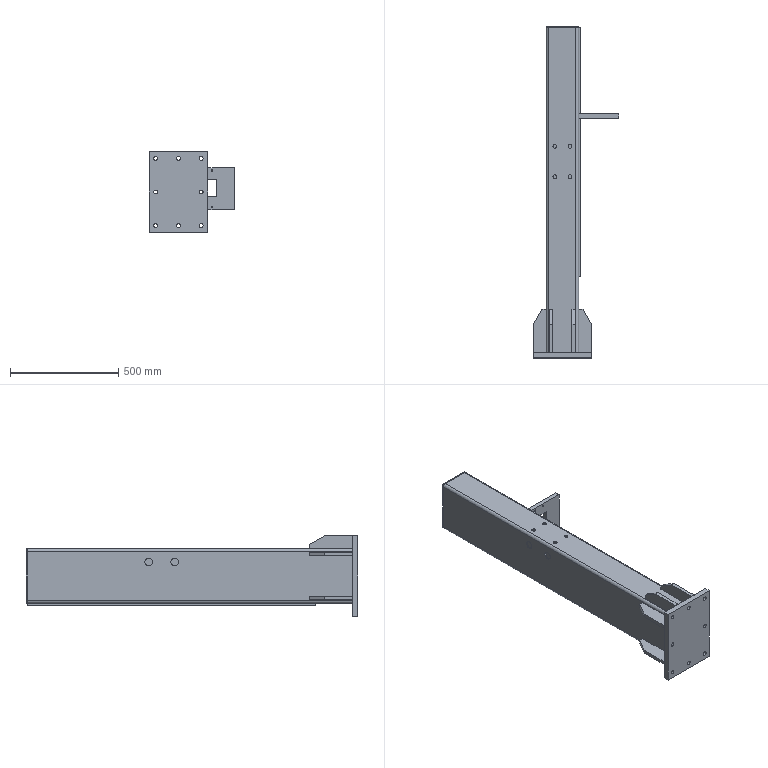Part | SolidWorks | features ICE 8, HoleWzd 4, Cut 2, MirrorSolid 2, Fillet 1, WeldMemberFeat 1, WeldmentFeature 1 | 12 solids | 205 faces | box 395 x 1530 x 370 mm | volume 12639229 mm3 | cylinder 106 | plane 99 | commonest cylinder face diameters 12 x52 17.5 x24 7 x8 25.2 x8 12.6 x4 15.5 x4